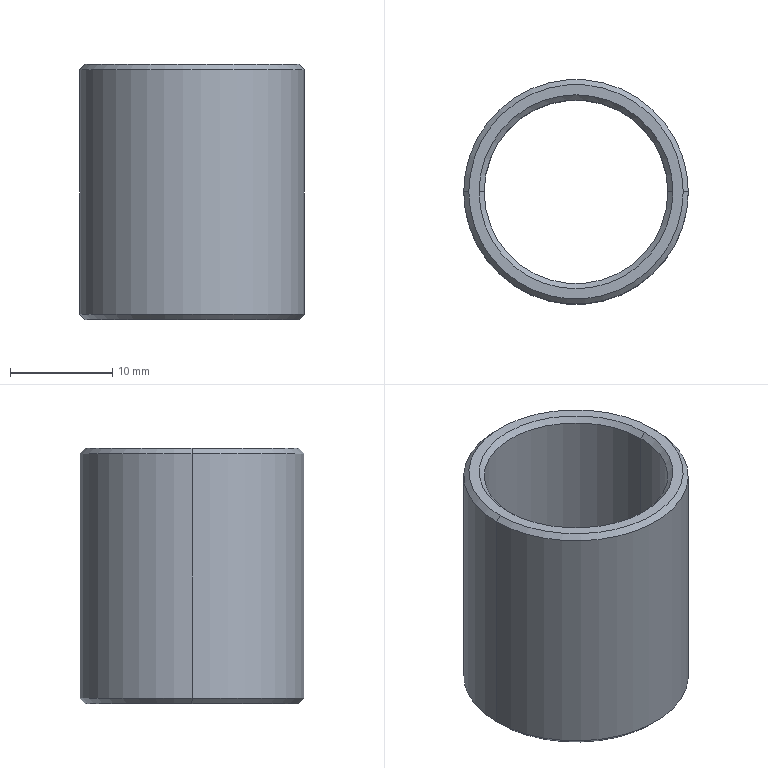Part | SolidWorks | features Chamfer 1, Extrusion 1 | 1 solid | 14 faces | box 22 x 22 x 25 mm | volume 3110 mm3 | cone 8 | cylinder 4 | plane 2 | commonest cylinder face diameters 18 x2 22 x2
STEP:
#1=CARTESIAN_POINT('',(-10.5,0.,0.));
#2=VERTEX_POINT('',#1);
#3=CARTESIAN_POINT('',(10.5,0.,0.));
#4=VERTEX_POINT('',#3);
#5=CARTESIAN_POINT('',(0.,0.,0.));
#6=DIRECTION('',(0.,0.,-1.));
#7=DIRECTION('',(1.,0.,0.));
#8=AXIS2_PLACEMENT_3D('',#5,#6,#7);
#9=CIRCLE('',#8,10.5);
#10=EDGE_CURVE('',#2,#4,#9,.T.);
#11=ORIENTED_EDGE('',*,*,#10,.F.);
#12=CARTESIAN_POINT('',(-11.,0.,0.5));
#13=VERTEX_POINT('',#12);
#14=CARTESIAN_POINT('',(-11.,0.,0.5));
#15=DIRECTION('',(-0.7071,0.,0.7071));
#16=VECTOR('',#15,1000.);
#17=LINE('',#14,#16);
#18=EDGE_CURVE('',#2,#13,#17,.T.);
#19=ORIENTED_EDGE('',*,*,#18,.T.);
#20=CARTESIAN_POINT('',(11.,0.,0.5));
#21=VERTEX_POINT('',#20);
#22=CARTESIAN_POINT('',(0.,0.,0.5));
#23=DIRECTION('',(0.,0.,1.));
#24=DIRECTION('',(1.,0.,0.));
#25=AXIS2_PLACEMENT_3D('',#22,#23,#24);
#26=CIRCLE('',#25,11.);
#27=EDGE_CURVE('',#21,#13,#26,.T.);
#28=ORIENTED_EDGE('',*,*,#27,.F.);
#29=CARTESIAN_POINT('',(11.,0.,0.5));
#30=DIRECTION('',(0.7071,0.,0.7071));
#31=VECTOR('',#30,1000.);
#32=LINE('',#29,#31);
#33=EDGE_CURVE('',#4,#21,#32,.T.);
#34=ORIENTED_EDGE('',*,*,#33,.F.);
#35=EDGE_LOOP('',(#11,#19,#28,#34));
#36=FACE_OUTER_BOUND('',#35,.T.);
#37=CARTESIAN_POINT('',(0.,0.,0.5));
#38=DIRECTION('',(0.,0.,1.));
#39=DIRECTION('',(1.,0.,0.));
#40=AXIS2_PLACEMENT_3D('',#37,#38,#39);
#41=CONICAL_SURFACE('',#40,11.,0.7854);
#42=ADVANCED_FACE('',(#36),#41,.T.);
#43=CARTESIAN_POINT('',(9.,0.,0.5));
#44=VERTEX_POINT('',#43);
#45=CARTESIAN_POINT('',(-9.,0.,0.5));
#46=VERTEX_POINT('',#45);
#47=CARTESIAN_POINT('',(0.,0.,0.5));
#48=DIRECTION('',(0.,0.,-1.));
#49=DIRECTION('',(1.,0.,0.));
#50=AXIS2_PLACEMENT_3D('',#47,#48,#49);
#51=CIRCLE('',#50,9.);
#52=EDGE_CURVE('',#44,#46,#51,.T.);
#53=ORIENTED_EDGE('',*,*,#52,.F.);
#54=CARTESIAN_POINT('',(9.5,0.,0.));
#55=VERTEX_POINT('',#54);
#56=CARTESIAN_POINT('',(9.5,0.,0.));
#57=DIRECTION('',(0.7071,0.,-0.7071));
#58=VECTOR('',#57,1000.);
#59=LINE('',#56,#58);
#60=EDGE_CURVE('',#44,#55,#59,.T.);
#61=ORIENTED_EDGE('',*,*,#60,.T.);
#62=CARTESIAN_POINT('',(-9.5,0.,0.));
#63=VERTEX_POINT('',#62);
#64=CARTESIAN_POINT('',(0.,0.,0.));
#65=DIRECTION('',(0.,0.,1.));
#66=DIRECTION('',(1.,0.,0.));
#67=AXIS2_PLACEMENT_3D('',#64,#65,#66);
#68=CIRCLE('',#67,9.5);
#69=EDGE_CURVE('',#63,#55,#68,.T.);
#70=ORIENTED_EDGE('',*,*,#69,.F.);
#71=CARTESIAN_POINT('',(-9.5,0.,0.));
#72=DIRECTION('',(-0.7071,0.,-0.7071));
#73=VECTOR('',#72,1000.);
#74=LINE('',#71,#73);
#75=EDGE_CURVE('',#46,#63,#74,.T.);
#76=ORIENTED_EDGE('',*,*,#75,.F.);
#77=EDGE_LOOP('',(#53,#61,#70,#76));
#78=FACE_OUTER_BOUND('',#77,.T.);
#79=CARTESIAN_POINT('',(0.,0.,0.));
#80=DIRECTION('',(0.,0.,-1.));
#81=DIRECTION('',(-1.,0.,0.));
#82=AXIS2_PLACEMENT_3D('',#79,#80,#81);
#83=CONICAL_SURFACE('',#82,9.5,0.7854);
#84=ADVANCED_FACE('',(#78),#83,.F.);
#85=CARTESIAN_POINT('',(10.5,0.,25.));
#86=VERTEX_POINT('',#85);
#87=CARTESIAN_POINT('',(-10.5,0.,25.));
#88=VERTEX_POINT('',#87);
#89=CARTESIAN_POINT('',(0.,0.,25.));
#90=DIRECTION('',(0.,0.,1.));
#91=DIRECTION('',(1.,0.,0.));
#92=AXIS2_PLACEMENT_3D('',#89,#90,#91);
#93=CIRCLE('',#92,10.5);
#94=EDGE_CURVE('',#86,#88,#93,.T.);
#95=ORIENTED_EDGE('',*,*,#94,.F.);
#96=CARTESIAN_POINT('',(11.,0.,24.5));
#97=VERTEX_POINT('',#96);
#98=CARTESIAN_POINT('',(10.5,0.,25.));
#99=DIRECTION('',(0.7071,0.,-0.7071));
#100=VECTOR('',#99,1000.);
#101=LINE('',#98,#100);
#102=EDGE_CURVE('',#86,#97,#101,.T.);
#103=ORIENTED_EDGE('',*,*,#102,.T.);
#104=CARTESIAN_POINT('',(-11.,0.,24.5));
#105=VERTEX_POINT('',#104);
#106=CARTESIAN_POINT('',(0.,0.,24.5));
#107=DIRECTION('',(0.,0.,-1.));
#108=DIRECTION('',(1.,0.,0.));
#109=AXIS2_PLACEMENT_3D('',#106,#107,#108);
#110=CIRCLE('',#109,11.);
#111=EDGE_CURVE('',#105,#97,#110,.T.);
#112=ORIENTED_EDGE('',*,*,#111,.F.);
#113=CARTESIAN_POINT('',(-10.5,0.,25.));
#114=DIRECTION('',(-0.7071,0.,-0.7071));
#115=VECTOR('',#114,1000.);
#116=LINE('',#113,#115);
#117=EDGE_CURVE('',#88,#105,#116,.T.);
#118=ORIENTED_EDGE('',*,*,#117,.F.);
#119=EDGE_LOOP('',(#95,#103,#112,#118));
#120=FACE_OUTER_BOUND('',#119,.T.);
#121=CARTESIAN_POINT('',(0.,0.,25.));
#122=DIRECTION('',(0.,0.,-1.));
#123=DIRECTION('',(-1.,0.,0.));
#124=AXIS2_PLACEMENT_3D('',#121,#122,#123);
#125=CONICAL_SURFACE('',#124,10.5,0.7854);
#126=ADVANCED_FACE('',(#120),#125,.T.);
#127=CARTESIAN_POINT('',(-9.,0.,24.5));
#128=VERTEX_POINT('',#127);
#129=CARTESIAN_POINT('',(9.,0.,24.5));
#130=VERTEX_POINT('',#129);
#131=CARTESIAN_POINT('',(0.,0.,24.5));
#132=DIRECTION('',(0.,0.,1.));
#133=DIRECTION('',(1.,0.,0.));
#134=AXIS2_PLACEMENT_3D('',#131,#132,#133);
#135=CIRCLE('',#134,9.);
#136=EDGE_CURVE('',#128,#130,#135,.T.);
#137=ORIENTED_EDGE('',*,*,#136,.F.);
#138=CARTESIAN_POINT('',(-9.5,0.,25.));
#139=VERTEX_POINT('',#138);
#140=CARTESIAN_POINT('',(-9.,0.,24.5));
#141=DIRECTION('',(-0.7071,0.,0.7071));
#142=VECTOR('',#141,1000.);
#143=LINE('',#140,#142);
#144=EDGE_CURVE('',#128,#139,#143,.T.);
#145=ORIENTED_EDGE('',*,*,#144,.T.);
#146=CARTESIAN_POINT('',(9.5,0.,25.));
#147=VERTEX_POINT('',#146);
#148=CARTESIAN_POINT('',(0.,0.,25.));
#149=DIRECTION('',(0.,0.,-1.));
#150=DIRECTION('',(1.,0.,0.));
#151=AXIS2_PLACEMENT_3D('',#148,#149,#150);
#152=CIRCLE('',#151,9.5);
#153=EDGE_CURVE('',#147,#139,#152,.T.);
#154=ORIENTED_EDGE('',*,*,#153,.F.);
#155=CARTESIAN_POINT('',(9.,0.,24.5));
#156=DIRECTION('',(0.7071,0.,0.7071));
#157=VECTOR('',#156,1000.);
#158=LINE('',#155,#157);
#159=EDGE_CURVE('',#130,#147,#158,.T.);
#160=ORIENTED_EDGE('',*,*,#159,.F.);
#161=EDGE_LOOP('',(#137,#145,#154,#160));
#162=FACE_OUTER_BOUND('',#161,.T.);
#163=CARTESIAN_POINT('',(0.,0.,24.5));
#164=DIRECTION('',(0.,0.,1.));
#165=DIRECTION('',(1.,0.,0.));
#166=AXIS2_PLACEMENT_3D('',#163,#164,#165);
#167=CONICAL_SURFACE('',#166,9.,0.7854);
#168=ADVANCED_FACE('',(#162),#167,.F.);
#169=ORIENTED_EDGE('',*,*,#136,.T.);
#170=CARTESIAN_POINT('',(9.,0.,25.));
#171=DIRECTION('',(0.,0.,-1.));
#172=VECTOR('',#171,1000.);
#173=LINE('',#170,#172);
#174=EDGE_CURVE('',#130,#44,#173,.T.);
#175=ORIENTED_EDGE('',*,*,#174,.T.);
#176=ORIENTED_EDGE('',*,*,#52,.T.);
#177=CARTESIAN_POINT('',(-9.,0.,25.));
#178=DIRECTION('',(0.,0.,-1.));
#179=VECTOR('',#178,1000.);
#180=LINE('',#177,#179);
#181=EDGE_CURVE('',#128,#46,#180,.T.);
#182=ORIENTED_EDGE('',*,*,#181,.F.);
#183=EDGE_LOOP('',(#169,#175,#176,#182));
#184=FACE_OUTER_BOUND('',#183,.T.);
#185=CARTESIAN_POINT('',(0.,0.,25.));
#186=DIRECTION('',(0.,0.,-1.));
#187=DIRECTION('',(-1.,0.,0.));
#188=AXIS2_PLACEMENT_3D('',#185,#186,#187);
#189=CYLINDRICAL_SURFACE('',#188,9.);
#190=ADVANCED_FACE('',(#184),#189,.F.);
#191=ORIENTED_EDGE('',*,*,#111,.T.);
#192=CARTESIAN_POINT('',(11.,0.,25.));
#193=DIRECTION('',(0.,0.,-1.));
#194=VECTOR('',#193,1000.);
#195=LINE('',#192,#194);
#196=EDGE_CURVE('',#97,#21,#195,.T.);
#197=ORIENTED_EDGE('',*,*,#196,.T.);
#198=ORIENTED_EDGE('',*,*,#27,.T.);
#199=CARTESIAN_POINT('',(-11.,0.,25.));
#200=DIRECTION('',(0.,0.,-1.));
#201=VECTOR('',#200,1000.);
#202=LINE('',#199,#201);
#203=EDGE_CURVE('',#105,#13,#202,.T.);
#204=ORIENTED_EDGE('',*,*,#203,.F.);
#205=EDGE_LOOP('',(#191,#197,#198,#204));
#206=FACE_OUTER_BOUND('',#205,.T.);
#207=CARTESIAN_POINT('',(0.,0.,25.));
#208=DIRECTION('',(0.,0.,-1.));
#209=DIRECTION('',(-1.,0.,0.));
#210=AXIS2_PLACEMENT_3D('',#207,#208,#209);
#211=CYLINDRICAL_SURFACE('',#210,11.);
#212=ADVANCED_FACE('',(#206),#211,.T.);
#213=ORIENTED_EDGE('',*,*,#153,.T.);
#214=CARTESIAN_POINT('',(0.,0.,25.));
#215=DIRECTION('',(0.,0.,-1.));
#216=DIRECTION('',(1.,0.,0.));
#217=AXIS2_PLACEMENT_3D('',#214,#215,#216);
#218=CIRCLE('',#217,9.5);
#219=EDGE_CURVE('',#139,#147,#218,.T.);
#220=ORIENTED_EDGE('',*,*,#219,.T.);
#221=EDGE_LOOP('',(#213,#220));
#222=FACE_BOUND('',#221,.T.);
#223=CARTESIAN_POINT('',(0.,0.,25.));
#224=DIRECTION('',(0.,0.,1.));
#225=DIRECTION('',(1.,0.,0.));
#226=AXIS2_PLACEMENT_3D('',#223,#224,#225);
#227=CIRCLE('',#226,10.5);
#228=EDGE_CURVE('',#88,#86,#227,.T.);
#229=ORIENTED_EDGE('',*,*,#228,.T.);
#230=ORIENTED_EDGE('',*,*,#94,.T.);
#231=EDGE_LOOP('',(#229,#230));
#232=FACE_OUTER_BOUND('',#231,.T.);
#233=CARTESIAN_POINT('',(0.,0.,25.));
#234=DIRECTION('',(0.,0.,1.));
#235=DIRECTION('',(1.,0.,0.));
#236=AXIS2_PLACEMENT_3D('',#233,#234,#235);
#237=PLANE('',#236);
#238=ADVANCED_FACE('',(#222,#232),#237,.T.);
#239=ORIENTED_EDGE('',*,*,#69,.T.);
#240=CARTESIAN_POINT('',(0.,0.,0.));
#241=DIRECTION('',(0.,0.,1.));
#242=DIRECTION('',(1.,0.,0.));
#243=AXIS2_PLACEMENT_3D('',#240,#241,#242);
#244=CIRCLE('',#243,9.5);
#245=EDGE_CURVE('',#55,#63,#244,.T.);
#246=ORIENTED_EDGE('',*,*,#245,.T.);
#247=EDGE_LOOP('',(#239,#246));
#248=FACE_BOUND('',#247,.T.);
#249=CARTESIAN_POINT('',(0.,0.,0.));
#250=DIRECTION('',(0.,0.,-1.));
#251=DIRECTION('',(1.,0.,0.));
#252=AXIS2_PLACEMENT_3D('',#249,#250,#251);
#253=CIRCLE('',#252,10.5);
#254=EDGE_CURVE('',#4,#2,#253,.T.);
#255=ORIENTED_EDGE('',*,*,#254,.T.);
#256=ORIENTED_EDGE('',*,*,#10,.T.);
#257=EDGE_LOOP('',(#255,#256));
#258=FACE_OUTER_BOUND('',#257,.T.);
#259=CARTESIAN_POINT('',(0.,0.,0.));
#260=DIRECTION('',(0.,0.,1.));
#261=DIRECTION('',(1.,0.,0.));
#262=AXIS2_PLACEMENT_3D('',#259,#260,#261);
#263=PLANE('',#262);
#264=ADVANCED_FACE('',(#248,#258),#263,.F.);
#265=ORIENTED_EDGE('',*,*,#196,.F.);
#266=CARTESIAN_POINT('',(0.,0.,24.5));
#267=DIRECTION('',(0.,0.,-1.));
#268=DIRECTION('',(1.,0.,0.));
#269=AXIS2_PLACEMENT_3D('',#266,#267,#268);
#270=CIRCLE('',#269,11.);
#271=EDGE_CURVE('',#97,#105,#270,.T.);
#272=ORIENTED_EDGE('',*,*,#271,.T.);
#273=ORIENTED_EDGE('',*,*,#203,.T.);
#274=CARTESIAN_POINT('',(0.,0.,0.5));
#275=DIRECTION('',(0.,0.,1.));
#276=DIRECTION('',(1.,0.,0.));
#277=AXIS2_PLACEMENT_3D('',#274,#275,#276);
#278=CIRCLE('',#277,11.);
#279=EDGE_CURVE('',#13,#21,#278,.T.);
#280=ORIENTED_EDGE('',*,*,#279,.T.);
#281=EDGE_LOOP('',(#265,#272,#273,#280));
#282=FACE_OUTER_BOUND('',#281,.T.);
#283=CARTESIAN_POINT('',(0.,0.,25.));
#284=DIRECTION('',(0.,0.,-1.));
#285=DIRECTION('',(-1.,0.,0.));
#286=AXIS2_PLACEMENT_3D('',#283,#284,#285);
#287=CYLINDRICAL_SURFACE('',#286,11.);
#288=ADVANCED_FACE('',(#282),#287,.T.);
#289=ORIENTED_EDGE('',*,*,#174,.F.);
#290=CARTESIAN_POINT('',(0.,0.,24.5));
#291=DIRECTION('',(0.,0.,1.));
#292=DIRECTION('',(1.,0.,0.));
#293=AXIS2_PLACEMENT_3D('',#290,#291,#292);
#294=CIRCLE('',#293,9.);
#295=EDGE_CURVE('',#130,#128,#294,.T.);
#296=ORIENTED_EDGE('',*,*,#295,.T.);
#297=ORIENTED_EDGE('',*,*,#181,.T.);
#298=CARTESIAN_POINT('',(0.,0.,0.5));
#299=DIRECTION('',(0.,0.,-1.));
#300=DIRECTION('',(1.,0.,0.));
#301=AXIS2_PLACEMENT_3D('',#298,#299,#300);
#302=CIRCLE('',#301,9.);
#303=EDGE_CURVE('',#46,#44,#302,.T.);
#304=ORIENTED_EDGE('',*,*,#303,.T.);
#305=EDGE_LOOP('',(#289,#296,#297,#304));
#306=FACE_OUTER_BOUND('',#305,.T.);
#307=CARTESIAN_POINT('',(0.,0.,25.));
#308=DIRECTION('',(0.,0.,-1.));
#309=DIRECTION('',(-1.,0.,0.));
#310=AXIS2_PLACEMENT_3D('',#307,#308,#309);
#311=CYLINDRICAL_SURFACE('',#310,9.);
#312=ADVANCED_FACE('',(#306),#311,.F.);
#313=ORIENTED_EDGE('',*,*,#144,.F.);
#314=ORIENTED_EDGE('',*,*,#295,.F.);
#315=ORIENTED_EDGE('',*,*,#159,.T.);
#316=ORIENTED_EDGE('',*,*,#219,.F.);
#317=EDGE_LOOP('',(#313,#314,#315,#316));
#318=FACE_OUTER_BOUND('',#317,.T.);
#319=CARTESIAN_POINT('',(0.,0.,24.5));
#320=DIRECTION('',(0.,0.,1.));
#321=DIRECTION('',(1.,0.,0.));
#322=AXIS2_PLACEMENT_3D('',#319,#320,#321);
#323=CONICAL_SURFACE('',#322,9.,0.7854);
#324=ADVANCED_FACE('',(#318),#323,.F.);
#325=ORIENTED_EDGE('',*,*,#102,.F.);
#326=ORIENTED_EDGE('',*,*,#228,.F.);
#327=ORIENTED_EDGE('',*,*,#117,.T.);
#328=ORIENTED_EDGE('',*,*,#271,.F.);
#329=EDGE_LOOP('',(#325,#326,#327,#328));
#330=FACE_OUTER_BOUND('',#329,.T.);
#331=CARTESIAN_POINT('',(0.,0.,25.));
#332=DIRECTION('',(0.,0.,-1.));
#333=DIRECTION('',(-1.,0.,0.));
#334=AXIS2_PLACEMENT_3D('',#331,#332,#333);
#335=CONICAL_SURFACE('',#334,10.5,0.7854);
#336=ADVANCED_FACE('',(#330),#335,.T.);
#337=ORIENTED_EDGE('',*,*,#60,.F.);
#338=ORIENTED_EDGE('',*,*,#303,.F.);
#339=ORIENTED_EDGE('',*,*,#75,.T.);
#340=ORIENTED_EDGE('',*,*,#245,.F.);
#341=EDGE_LOOP('',(#337,#338,#339,#340));
#342=FACE_OUTER_BOUND('',#341,.T.);
#343=CARTESIAN_POINT('',(0.,0.,0.));
#344=DIRECTION('',(0.,0.,-1.));
#345=DIRECTION('',(-1.,0.,0.));
#346=AXIS2_PLACEMENT_3D('',#343,#344,#345);
#347=CONICAL_SURFACE('',#346,9.5,0.7854);
#348=ADVANCED_FACE('',(#342),#347,.F.);
#349=ORIENTED_EDGE('',*,*,#18,.F.);
#350=ORIENTED_EDGE('',*,*,#254,.F.);
#351=ORIENTED_EDGE('',*,*,#33,.T.);
#352=ORIENTED_EDGE('',*,*,#279,.F.);
#353=EDGE_LOOP('',(#349,#350,#351,#352));
#354=FACE_OUTER_BOUND('',#353,.T.);
#355=CARTESIAN_POINT('',(0.,0.,0.5));
#356=DIRECTION('',(0.,0.,1.));
#357=DIRECTION('',(1.,0.,0.));
#358=AXIS2_PLACEMENT_3D('',#355,#356,#357);
#359=CONICAL_SURFACE('',#358,11.,0.7854);
#360=ADVANCED_FACE('',(#354),#359,.T.);
#361=CLOSED_SHELL('',(#42,#84,#126,#168,#190,#212,#238,#264,#288,#312,#324,#336,#348,#360));
#362=MANIFOLD_SOLID_BREP('',#361);
#363=CARTESIAN_POINT('',(0.,0.,0.));
#364=DIRECTION('',(0.,0.,1.));
#365=DIRECTION('',(1.,0.,0.));
#366=AXIS2_PLACEMENT_3D('',#363,#364,#365);
#367=(LENGTH_UNIT()NAMED_UNIT(*)SI_UNIT(.MILLI.,.METRE.));
#368=UNCERTAINTY_MEASURE_WITH_UNIT(LENGTH_MEASURE(0.00001),#367,'','');
#369=(NAMED_UNIT(*)PLANE_ANGLE_UNIT()SI_UNIT($,.RADIAN.));
#370=(NAMED_UNIT(*)SI_UNIT($,.STERADIAN.)SOLID_ANGLE_UNIT());
#371=(GEOMETRIC_REPRESENTATION_CONTEXT(3)GLOBAL_UNCERTAINTY_ASSIGNED_CONTEXT((#368))GLOBAL_UNIT_ASSIGNED_CONTEXT((#367,#369,#370))REPRESENTATION_CONTEXT('',''));
#372=ADVANCED_BREP_SHAPE_REPRESENTATION('',(#362,#366),#371);